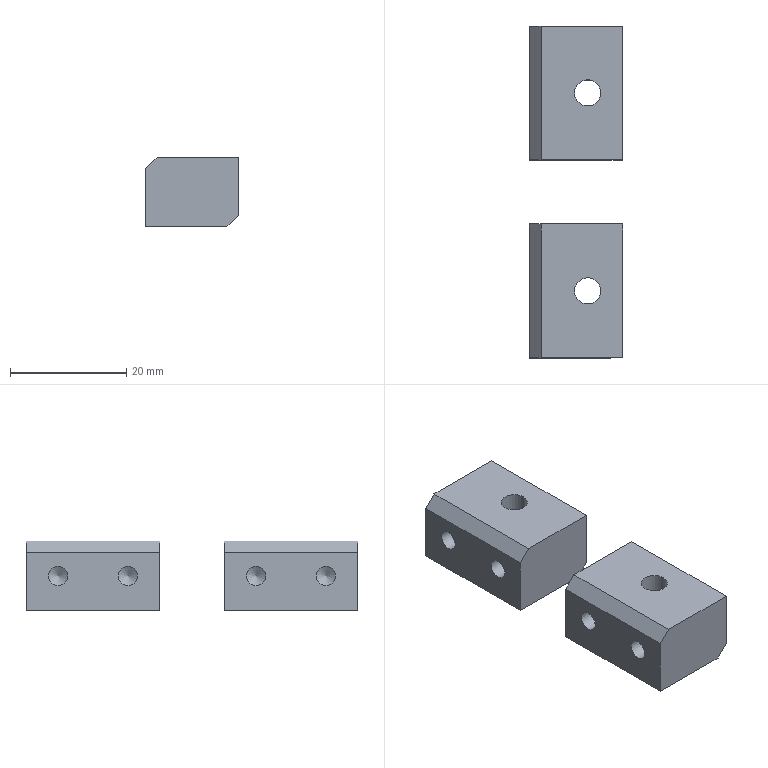NC program | NX | posted by the shop | part box 16 x 57 x 12 mm
Whole program:
%
O0001
(Machine time: 79.98 MIN)
(===Total Tool:6===)
(T1=D80R0.8 fly cutter D=80.  R=0.8  D-  H01 Z=0.    )
(T9=D10     D=10.  R=0.   D-  H09 Z=-16.3 )
(T2=D6 chamfer tool   D=6.   R=0.   D-  H02 Z=-2.7  )
(T13=drill 3.3  D=3.3  DR_a=118 D-  H13 Z=-9.09 )
(T21=M4X0.7 D=3.3  DR_a=180 D-  H21 Z=-6.1  )
(T10=D10-J  D=10.  R=0.   D10 H10 Z=-16.  )
G80 G90 G17 G49 G40
G91 G28 Z0
M01
N1 T01 M06
(D80R0.8 fly cutter  D=80. R=0.8 H=01 ce=0.20 di=0.10)
G00 G90 G54 X-73.5 Y0.0 M03 S4000
G43 H01 Z20.
M08
Z2.1
G01 Z.1 F3000.
X-68.5
X68.5
X73.5
Z2.1
G00 Z20.
G00 G90 X-73.5 Y0.0 M03 S4000
Z20.
Z2.
G01 Z0.0 F1000.
X-68.5
X68.5
X73.5
Z2.
G00 Z20.
G91 G28 Z0.0
M05
M09
G91 G28 Z0.0
M01
N2 T09 M06
(D10  D=10. R=0. H=09 ce=0.10 di=0.10)
G00 G90 G54 X-24.988 Y-9.724 M03 S8000
G43 H09 Z20.
M08
Z1.
G01 X-29.064 Z.786 F4000.
X-30.559 Y-9.324 Z.705
X-31.865 Y-8.493 Z.624
X-32.86 Y-7.309 Z.543
X-33.454 Y-5.88 Z.462
X-33.577 Y-4.959 Z.413
X-33.6 Y-4.582 Z.394
Y6.554 Z-.19
X-33.266 Y7.898 Z-.263
X-32.584 Y9.104 Z-.335
X-31.604 Y10.084 Z-.408
X-30.398 Y10.766 Z-.481
X-29.054 Y11.1 Z-.553
X-28.5 Z-.582
X-5.5
G02 X-.4 Y6. I0.0 J-5.1
G01 Y-4.582
G02 X-1.931 Y-8.258 I-5.264 J.037
X-5.457 Y-9.724 I-3.525 J3.506
G01 X-28.512
G02 X-33.527 Y-5.333 I0.0 J5.059
X-33.6 Y-4.582 I10.531 J1.404
G01 Y6.
G02 X-28.5 Y11.1 I5.1 J0.0
G01 X-17.392 Z-1.164
X-5.5
G02 X-.4 Y6. I0.0 J-5.1
G01 Y-5.164
G02 X-1.931 Y-8.84 I-5.262 J.036
X-5.457 Y-10.306 I-3.526 J3.507
G01 X-28.516
G02 X-33.546 Y-5.729 I0.0 J5.053
G01 X-33.6 Y-5.164
Y6.
G02 X-28.5 Y11.1 I5.1 J0.0
G01 X-17.392 Z-1.746
X-5.5
G02 X-.4 Y6. I0.0 J-5.1
G01 Y-5.746
Y-5.767
G02 X-5.5 Y-10.888 I-5.121 J0.0
G01 X-28.5
G02 X-33.6 Y-5.767 I.021 J5.121
G01 Y-5.746
Y6.
G02 X-28.5 Y11.1 I5.1 J0.0
G01 X-17.392 Z-2.329
X-5.5
G02 X-.4 Y6. I0.0 J-5.1
G01 Y-6.
G02 X-5.5 Y-11.1 I-5.1 J0.0
G01 X-28.5
G02 X-33.6 Y-6. I0.0 J5.1
G01 Y6.
G02 X-28.5 Y11.1 I5.1 J0.0
G01 X-17.392 Z-2.911
X-5.5
G02 X-.4 Y6. I0.0 J-5.1
G01 Y-6.
G02 X-5.5 Y-11.1 I-5.1 J0.0
G01 X-28.5
G02 X-33.6 Y-6. I0.0 J5.1
G01 Y6.
G02 X-28.5 Y11.1 I5.1 J0.0
G01 X-17.392 Z-3.493
X-5.5
G02 X-.4 Y6. I0.0 J-5.1
G01 Y-6.
G02 X-5.5 Y-11.1 I-5.1 J0.0
G01 X-28.5
G02 X-33.6 Y-6. I0.0 J5.1
G01 Y6.
G02 X-28.5 Y11.1 I5.1 J0.0
G01 X-17.392 Z-4.075
X-5.5
G02 X-.4 Y6. I0.0 J-5.1
G01 Y-6.
G02 X-5.5 Y-11.1 I-5.1 J0.0
G01 X-28.5
G02 X-33.6 Y-6. I0.0 J5.1
G01 Y6.
G02 X-28.5 Y11.1 I5.1 J0.0
G01 X-17.392 Z-4.657
X-5.5
G02 X-.4 Y6. I0.0 J-5.1
G01 Y-6.
G02 X-5.5 Y-11.1 I-5.1 J0.0
G01 X-28.5
G02 X-33.6 Y-6. I0.0 J5.1
G01 Y6.
G02 X-28.5 Y11.1 I5.1 J0.0
G01 X-17.392 Z-5.239
X-5.5
G02 X-.4 Y6. I0.0 J-5.1
G01 Y-6.
G02 X-5.5 Y-11.1 I-5.1 J0.0
G01 X-28.5
G02 X-33.6 Y-6. I0.0 J5.1
G01 Y6.
G02 X-28.5 Y11.1 I5.1 J0.0
G01 X-17.392 Z-5.821
X-5.5
G02 X-.4 Y6. I0.0 J-5.1
G01 Y-6.
G02 X-5.5 Y-11.1 I-5.1 J0.0
G01 X-28.5
G02 X-33.6 Y-6. I0.0 J5.1
G01 Y6.
G02 X-28.5 Y11.1 I5.1 J0.0
G01 X-17.392 Z-6.404
X-5.5
G02 X-.4 Y6. I0.0 J-5.1
G01 Y-6.
G02 X-5.5 Y-11.1 I-5.1 J0.0
G01 X-28.5
G02 X-33.6 Y-6. I0.0 J5.1
G01 Y6.
G02 X-28.5 Y11.1 I5.1 J0.0
G01 X-17.392 Z-6.986
X-5.5
G02 X-.4 Y6. I0.0 J-5.1
G01 Y-6.
G02 X-5.5 Y-11.1 I-5.1 J0.0
G01 X-28.5
G02 X-33.6 Y-6. I0.0 J5.1
G01 Y6.
G02 X-28.5 Y11.1 I5.1 J0.0
G01 X-17.392 Z-7.568
X-5.5
G02 X-.4 Y6. I0.0 J-5.1
G01 Y-6.
G02 X-5.5 Y-11.1 I-5.1 J0.0
G01 X-28.5
G02 X-33.6 Y-6. I0.0 J5.1
G01 Y6.
G02 X-28.5 Y11.1 I5.1 J0.0
G01 X-17.392 Z-8.15
X-5.5
G02 X-.4 Y6. I0.0 J-5.1
G01 Y-6.
G02 X-5.5 Y-11.1 I-5.1 J0.0
G01 X-28.5
G02 X-33.6 Y-6. I0.0 J5.1
G01 Y6.
G02 X-28.5 Y11.1 I5.1 J0.0
G01 X-17.392 Z-8.732
X-5.5
G02 X-.4 Y6. I0.0 J-5.1
G01 Y-6.
G02 X-5.5 Y-11.1 I-5.1 J0.0
G01 X-28.5
G02 X-33.6 Y-6. I0.0 J5.1
G01 Y6.
G02 X-28.5 Y11.1 I5.1 J0.0
G01 X-17.392 Z-9.314
X-5.5
G02 X-.4 Y6. I0.0 J-5.1
G01 Y-6.
G02 X-5.5 Y-11.1 I-5.1 J0.0
G01 X-28.5
G02 X-33.6 Y-6. I0.0 J5.1
G01 Y6.
G02 X-28.5 Y11.1 I5.1 J0.0
G01 X-17.392 Z-9.896
X-5.5
G02 X-.4 Y6. I0.0 J-5.1
G01 Y-6.
G02 X-5.5 Y-11.1 I-5.1 J0.0
G01 X-28.5
G02 X-33.6 Y-6. I0.0 J5.1
G01 Y6.
G02 X-28.5 Y11.1 I5.1 J0.0
G01 X-17.392 Z-10.479
X-5.5
G02 X-.4 Y6. I0.0 J-5.1
G01 Y-6.
G02 X-5.5 Y-11.1 I-5.1 J0.0
G01 X-28.5
G02 X-33.6 Y-6. I0.0 J5.1
G01 Y6.
G02 X-28.5 Y11.1 I5.1 J0.0
G01 X-17.392 Z-11.061
X-5.5
G02 X-.4 Y6. I0.0 J-5.1
G01 Y-6.
G02 X-5.5 Y-11.1 I-5.1 J0.0
G01 X-28.5
G02 X-33.6 Y-6. I0.0 J5.1
G01 Y6.
G02 X-28.5 Y11.1 I5.1 J0.0
G01 X-17.392 Z-11.643
X-5.5
G02 X-.4 Y6. I0.0 J-5.1
G01 Y-6.
G02 X-5.5 Y-11.1 I-5.1 J0.0
G01 X-28.5
G02 X-33.6 Y-6. I0.0 J5.1
G01 Y6.
G02 X-28.5 Y11.1 I5.1 J0.0
G01 X-17.392 Z-12.225
X-5.5
G02 X-.4 Y6. I0.0 J-5.1
G01 Y-6.
G02 X-5.5 Y-11.1 I-5.1 J0.0
G01 X-28.5
G02 X-33.6 Y-6. I0.0 J5.1
G01 Y6.
G02 X-28.5 Y11.1 I5.1 J0.0
G01 X-17.392 Z-12.807
X-5.5
G02 X-.4 Y6. I0.0 J-5.1
G01 Y-6.
G02 X-5.5 Y-11.1 I-5.1 J0.0
G01 X-28.5
G02 X-33.6 Y-6. I0.0 J5.1
G01 Y6.
G02 X-28.5 Y11.1 I5.1 J0.0
G01 X-17.392 Z-13.389
X-5.5
G02 X-.4 Y6. I0.0 J-5.1
G01 Y-6.
G02 X-5.5 Y-11.1 I-5.1 J0.0
G01 X-28.5
G02 X-33.6 Y-6. I0.0 J5.1
G01 Y6.
G02 X-28.5 Y11.1 I5.1 J0.0
G01 X-17.392 Z-13.971
X-5.5
G02 X-.4 Y6. I0.0 J-5.1
G01 Y-6.
G02 X-5.5 Y-11.1 I-5.1 J0.0
G01 X-28.5
G02 X-33.6 Y-6. I0.0 J5.1
G01 Y6.
G02 X-28.5 Y11.1 I5.1 J0.0
G01 X-17.392 Z-14.554
X-5.5
G02 X-.4 Y6. I0.0 J-5.1
G01 Y-6.
G02 X-5.5 Y-11.1 I-5.1 J0.0
G01 X-28.5
G02 X-33.6 Y-6. I0.0 J5.1
G01 Y6.
G02 X-28.5 Y11.1 I5.1 J0.0
G01 X-21.835 Z-14.903
X-21.465 Z-14.922
X-21.095 Z-14.942
X-17.392 Z-15.136
X-5.5
G02 X-.4 Y6. I0.0 J-5.1
G01 Y-6.
G02 X-5.5 Y-11.1 I-5.1 J0.0
G01 X-28.5
G02 X-33.6 Y-6. I0.0 J5.1
G01 Y6.
G02 X-28.5 Y11.1 I5.1 J0.0
G01 X-21.835 Z-15.485
X-21.465 Z-15.504
X-21.095 Z-15.524
X-17.392 Z-15.718
X-5.5
G02 X-.4 Y6. I0.0 J-5.1
G01 Y-6.
G02 X-5.5 Y-11.1 I-5.1 J0.0
G01 X-28.5
G02 X-33.6 Y-6. I0.0 J5.1
G01 Y6.
G02 X-28.5 Y11.1 I5.1 J0.0
G01 X-21.835 Z-16.067
X-21.465 Z-16.087
X-21.095 Z-16.106
X-17.392 Z-16.3
X-5.5
G02 X-.4 Y6. I0.0 J-5.1
G01 Y-6.
G02 X-5.5 Y-11.1 I-5.1 J0.0
G01 X-28.5
G02 X-33.6 Y-6. I0.0 J5.1
G01 Y6.
G02 X-28.5 Y11.1 I5.1 J0.0
G01 X-17.392
Z-15.3
G00 Z20.
X9.012 Y-9.724
Z1.
G01 X4.936 Z.786
X3.442 Y-9.324 Z.705
X2.136 Y-8.494 Z.624
X1.14 Y-7.31 Z.543
X.546 Y-5.882 Z.462
X.423 Y-4.96 Z.413
X.4 Y-4.582 Z.394
Y6.554 Z-.19
X.734 Y7.898 Z-.263
X1.416 Y9.104 Z-.335
X2.396 Y10.084 Z-.408
X3.602 Y10.766 Z-.481
X4.946 Y11.1 Z-.553
X5.5 Z-.582
X28.5
G02 X33.6 Y6. I0.0 J-5.1
G01 Y-4.582
G02 X32.061 Y-8.265 I-5.276 J.042
X28.548 Y-9.724 I-3.513 J3.501
G01 X5.488
G02 X.473 Y-5.335 I0.0 J5.06
X.4 Y-4.582 I10.234 J1.371
G01 Y6.
G02 X5.5 Y11.1 I5.1 J0.0
G01 X16.608 Z-1.164
X28.5
G02 X33.6 Y6. I0.0 J-5.1
G01 Y-5.164
G02 X32.061 Y-8.847 I-5.274 J.041
X28.548 Y-10.306 I-3.514 J3.503
G01 X5.497
G02 X.452 Y-5.714 I0.0 J5.068
G01 X.4 Y-5.164
Y6.
G02 X5.5 Y11.1 I5.1 J0.0
G01 X16.608 Z-1.746
X28.5
G02 X33.6 Y6. I0.0 J-5.1
G01 Y-5.746
Y-5.767
G02 X28.5 Y-10.888 I-5.121 J0.0
G01 X5.5
G02 X.4 Y-5.767 I.021 J5.121
G01 Y-5.746
Y6.
G02 X5.5 Y11.1 I5.1 J0.0
G01 X16.608 Z-2.329
X28.5
G02 X33.6 Y6. I0.0 J-5.1
G01 Y-6.
G02 X28.5 Y-11.1 I-5.1 J0.0
G01 X5.5
G02 X.4 Y-6. I0.0 J5.1
G01 Y6.
G02 X5.5 Y11.1 I5.1 J0.0
G01 X16.608 Z-2.911
X28.5
G02 X33.6 Y6. I0.0 J-5.1
G01 Y-6.
G02 X28.5 Y-11.1 I-5.1 J0.0
G01 X5.5
G02 X.4 Y-6. I0.0 J5.1
G01 Y6.
G02 X5.5 Y11.1 I5.1 J0.0
G01 X16.608 Z-3.493
X28.5
G02 X33.6 Y6. I0.0 J-5.1
G01 Y-6.
G02 X28.5 Y-11.1 I-5.1 J0.0
G01 X5.5
G02 X.4 Y-6. I0.0 J5.1
G01 Y6.
G02 X5.5 Y11.1 I5.1 J0.0
G01 X16.608 Z-4.075
X28.5
G02 X33.6 Y6. I0.0 J-5.1
G01 Y-6.
G02 X28.5 Y-11.1 I-5.1 J0.0
G01 X5.5
G02 X.4 Y-6. I0.0 J5.1
G01 Y6.
G02 X5.5 Y11.1 I5.1 J0.0
G01 X16.608 Z-4.657
X28.5
G02 X33.6 Y6. I0.0 J-5.1
G01 Y-6.
G02 X28.5 Y-11.1 I-5.1 J0.0
G01 X5.5
G02 X.4 Y-6. I0.0 J5.1
G01 Y6.
G02 X5.5 Y11.1 I5.1 J0.0
G01 X16.608 Z-5.239
X28.5
G02 X33.6 Y6. I0.0 J-5.1
G01 Y-6.
G02 X28.5 Y-11.1 I-5.1 J0.0
G01 X5.5
G02 X.4 Y-6. I0.0 J5.1
G01 Y6.
G02 X5.5 Y11.1 I5.1 J0.0
G01 X16.608 Z-5.821
X28.5
G02 X33.6 Y6. I0.0 J-5.1
G01 Y-6.
G02 X28.5 Y-11.1 I-5.1 J0.0
G01 X5.5
G02 X.4 Y-6. I0.0 J5.1
G01 Y6.
G02 X5.5 Y11.1 I5.1 J0.0
G01 X16.608 Z-6.404
X28.5
G02 X33.6 Y6. I0.0 J-5.1
G01 Y-6.
G02 X28.5 Y-11.1 I-5.1 J0.0
G01 X5.5
G02 X.4 Y-6. I0.0 J5.1
G01 Y6.
G02 X5.5 Y11.1 I5.1 J0.0
G01 X16.608 Z-6.986
X28.5
G02 X33.6 Y6. I0.0 J-5.1
G01 Y-6.
G02 X28.5 Y-11.1 I-5.1 J0.0
G01 X5.5
G02 X.4 Y-6. I0.0 J5.1
G01 Y6.
G02 X5.5 Y11.1 I5.1 J0.0
G01 X16.608 Z-7.568
X28.5
G02 X33.6 Y6. I0.0 J-5.1
G01 Y-6.
G02 X28.5 Y-11.1 I-5.1 J0.0
G01 X5.5
G02 X.4 Y-6. I0.0 J5.1
G01 Y6.
G02 X5.5 Y11.1 I5.1 J0.0
G01 X16.608 Z-8.15
X28.5
G02 X33.6 Y6. I0.0 J-5.1
G01 Y-6.
G02 X28.5 Y-11.1 I-5.1 J0.0
G01 X5.5
G02 X.4 Y-6. I0.0 J5.1
G01 Y6.
G02 X5.5 Y11.1 I5.1 J0.0
G01 X16.608 Z-8.732
X28.5
G02 X33.6 Y6. I0.0 J-5.1
G01 Y-6.
G02 X28.5 Y-11.1 I-5.1 J0.0
G01 X5.5
G02 X.4 Y-6. I0.0 J5.1
G01 Y6.
G02 X5.5 Y11.1 I5.1 J0.0
G01 X16.608 Z-9.314
X28.5
G02 X33.6 Y6. I0.0 J-5.1
G01 Y-6.
G02 X28.5 Y-11.1 I-5.1 J0.0
G01 X5.5
G02 X.4 Y-6. I0.0 J5.1
G01 Y6.
G02 X5.5 Y11.1 I5.1 J0.0
G01 X16.608 Z-9.896
X28.5
G02 X33.6 Y6. I0.0 J-5.1
G01 Y-6.
G02 X28.5 Y-11.1 I-5.1 J0.0
G01 X5.5
G02 X.4 Y-6. I0.0 J5.1
G01 Y6.
G02 X5.5 Y11.1 I5.1 J0.0
G01 X16.608 Z-10.479
X28.5
G02 X33.6 Y6. I0.0 J-5.1
G01 Y-6.
G02 X28.5 Y-11.1 I-5.1 J0.0
G01 X5.5
G02 X.4 Y-6. I0.0 J5.1
G01 Y6.
G02 X5.5 Y11.1 I5.1 J0.0
G01 X16.608 Z-11.061
X28.5
G02 X33.6 Y6. I0.0 J-5.1
G01 Y-6.
G02 X28.5 Y-11.1 I-5.1 J0.0
G01 X5.5
G02 X.4 Y-6. I0.0 J5.1
G01 Y6.
G02 X5.5 Y11.1 I5.1 J0.0
G01 X16.608 Z-11.643
X28.5
G02 X33.6 Y6. I0.0 J-5.1
G01 Y-6.
G02 X28.5 Y-11.1 I-5.1 J0.0
G01 X5.5
G02 X.4 Y-6. I0.0 J5.1
G01 Y6.
G02 X5.5 Y11.1 I5.1 J0.0
G01 X16.608 Z-12.225
X28.5
G02 X33.6 Y6. I0.0 J-5.1
G01 Y-6.
G02 X28.5 Y-11.1 I-5.1 J0.0
G01 X5.5
G02 X.4 Y-6. I0.0 J5.1
G01 Y6.
G02 X5.5 Y11.1 I5.1 J0.0
G01 X16.608 Z-12.807
X28.5
G02 X33.6 Y6. I0.0 J-5.1
G01 Y-6.
G02 X28.5 Y-11.1 I-5.1 J0.0
G01 X5.5
G02 X.4 Y-6. I0.0 J5.1
G01 Y6.
G02 X5.5 Y11.1 I5.1 J0.0
G01 X16.608 Z-13.389
X28.5
G02 X33.6 Y6. I0.0 J-5.1
G01 Y-6.
G02 X28.5 Y-11.1 I-5.1 J0.0
G01 X5.5
G02 X.4 Y-6. I0.0 J5.1
G01 Y6.
G02 X5.5 Y11.1 I5.1 J0.0
G01 X16.608 Z-13.971
X28.5
G02 X33.6 Y6. I0.0 J-5.1
G01 Y-6.
G02 X28.5 Y-11.1 I-5.1 J0.0
G01 X5.5
G02 X.4 Y-6. I0.0 J5.1
G01 Y6.
G02 X5.5 Y11.1 I5.1 J0.0
G01 X16.608 Z-14.554
X28.5
G02 X33.6 Y6. I0.0 J-5.1
G01 Y-6.
G02 X28.5 Y-11.1 I-5.1 J0.0
G01 X5.5
G02 X.4 Y-6. I0.0 J5.1
G01 Y6.
G02 X5.5 Y11.1 I5.1 J0.0
G01 X16.608 Z-15.136
X28.5
G02 X33.6 Y6. I0.0 J-5.1
G01 Y-6.
G02 X28.5 Y-11.1 I-5.1 J0.0
G01 X5.5
G02 X.4 Y-6. I0.0 J5.1
G01 Y6.
G02 X5.5 Y11.1 I5.1 J0.0
G01 X16.608 Z-15.718
X28.5
G02 X33.6 Y6. I0.0 J-5.1
G01 Y-6.
G02 X28.5 Y-11.1 I-5.1 J0.0
G01 X5.5
G02 X.4 Y-6. I0.0 J5.1
G01 Y6.
G02 X5.5 Y11.1 I5.1 J0.0
G01 X16.608 Z-16.3
X28.5
G02 X33.6 Y6. I0.0 J-5.1
G01 Y-6.
G02 X28.5 Y-11.1 I-5.1 J0.0
G01 X5.5
G02 X.4 Y-6. I0.0 J5.1
G01 Y6.
G02 X5.5 Y11.1 I5.1 J0.0
G01 X16.608
Z-15.3
G00 Z20.
G00 G90 X-.001 Y-13.218 M03 S7000
Z10.878
Z.359
G01 Z-.141 F4500.
X.572 Y-9.233
X-4.428 Y-9.24
X-5.5 Y-9.241
X-29.5
X-29.572 Y-9.239
Y-9.312 Z-.212
Y-9.381 Z-.283
X-29.5 Y-9.383
X-5.5
X-4.428 Y-9.381
Y-9.454 Z-.354
X-4.427 Y-9.523 Z-.424
X-5.5 Y-9.524
X-29.5
X-29.572 Y-9.522
Y-9.595 Z-.495
X-29.573 Y-9.663 Z-.566
X-29.5 Y-9.666
X-5.5
X-4.427 Y-9.664
Y-9.736 Z-.636
Y-9.806 Z-.707
X-5.5 Y-9.807
X-29.5
X-29.573 Y-9.805
Y-9.878 Z-.778
Y-9.946 Z-.849
X-29.5 Y-9.949
X-5.5
X-4.427 Y-9.947
Y-10.019 Z-.919
Y-10.089 Z-.99
X-5.5 Y-10.09
X-29.5
X-29.573 Y-10.088
Y-10.161 Z-1.061
Y-10.229 Z-1.131
X-29.5 Y-10.231
X-5.5
X-4.427 Y-10.23
Y-10.302 Z-1.202
Y-10.371 Z-1.273
X-5.5 Y-10.373
X-29.5
X-29.573 Y-10.371
Y-10.444 Z-1.344
Y-10.512 Z-1.414
X-29.5 Y-10.514
X-5.5
X-4.427 Y-10.513
Y-10.585 Z-1.485
Y-10.654 Z-1.556
X-5.5 Y-10.656
X-29.5
X-29.572 Y-10.653
Y-10.711 Z-1.611
Y-10.764 Z-1.667
X-29.5 Y-10.767
X-5.5
X-4.428 Y-10.765
Y-10.822 Z-1.722
Y-10.876 Z-1.778
X-5.5 Y-10.878
X-29.5
X-29.572 Y-10.876
Y-10.933 Z-1.833
Y-10.987 Z-1.889
X-29.5 Y-10.989
X-5.5
X-4.428 Y-10.987
Y-11.044 Z-1.944
Y-11.099 Z-2.
X-29.572 Y-11.098
G00 Z10.878
X38.446 Y-8.963
Z.359
G01 Z-.141
X29.572 Y-9.239
X29.5 Y-9.241
X5.5
X4.428 Y-9.24
Y-9.312 Z-.212
Y-9.381 Z-.283
X5.5 Y-9.383
X29.5
X29.572 Y-9.381
Y-9.454 Z-.354
Y-9.522 Z-.424
X29.5 Y-9.524
X5.5
X4.428 Y-9.523
X4.427 Y-9.595 Z-.495
Y-9.664 Z-.566
X5.5 Y-9.666
X29.5
X29.573 Y-9.663
Y-9.736 Z-.636
Y-9.805 Z-.707
X29.5 Y-9.807
X5.5
X4.427 Y-9.806
Y-9.878 Z-.778
Y-9.947 Z-.849
X5.5 Y-9.949
X29.5
X29.573 Y-9.946
Y-10.019 Z-.919
Y-10.088 Z-.99
X29.5 Y-10.09
X5.5
X4.427 Y-10.089
Y-10.161 Z-1.061
Y-10.23 Z-1.131
X5.5 Y-10.231
X29.5
X29.573 Y-10.229
Y-10.302 Z-1.202
Y-10.371 Z-1.273
X29.5 Y-10.373
X5.5
X4.427 Y-10.371
Y-10.444 Z-1.344
Y-10.513 Z-1.414
X5.5 Y-10.514
X29.5
X29.573 Y-10.512
X29.572 Y-10.585 Z-1.485
Y-10.653 Z-1.556
X29.5 Y-10.656
X5.5
X4.427 Y-10.654
X4.428 Y-10.711 Z-1.611
Y-10.765 Z-1.667
X5.5 Y-10.767
X29.5
X29.572 Y-10.764
Y-10.822 Z-1.722
Y-10.876 Z-1.778
X29.5 Y-10.878
X5.5
X4.428 Y-10.876
Y-10.933 Z-1.833
Y-10.987 Z-1.889
X5.5 Y-10.989
X29.5
X29.572 Y-10.987
Y-11.044 Z-1.944
Y-11.098 Z-2.
X29.5 Y-11.1
X4.729
X4.428 Y-11.099
G00 Z10.878
G91 G28 Z0.0
M05
M09
G91 G28 Z0.0
M01
N3 T02 M06
(D6 chamfer tool  D=6. R=0. H=02 ce=0.00 di=0.00)
G00 G90 G54 X-23. Y0.0 M03 S8000
G43 H02 Z20.
M08
G98 G81 X-23. Y0.0 Z-.8 R1. F500.
X-11.
X11.
X23.
G80
G00 Z20.
G91 G28 Z0.0
M05
M09
G91 G28 Z0.0
M01
N4 T13 M06
(Drill 3.3 D=3.3 DR_a=118 H=13)
G00 G90 G54 X-23. Y0.0 M03 S3000
G43 H13 Z20.
M08
G98 G83 X-23. Y0.0 Z-9.091 R1. F120. Q2.
X-11.
X11.
X23.
G80
G00 Z20.
G91 G28 Z0.0
M05
M09
G91 G28 Z0.0
M01
N5 T02 M06
(D6 chamfer tool  D=6. R=0. H=02 ce=0.00 di=0.00)
G00 G90 G54 X4.293 Y-4.461 M03 S8000
G43 H02 Z20.
M08
Z2.935
G01 Z-1.5 F3000.
X4.233 Y-4.289
X4.2 Y-4.
Y6.
G02 X5.5 Y7.3 I1.3 J0.0
G01 X28.5
G02 X29.8 Y6. I0.0 J-1.3
G01 Y-4.
X29.767 Y-4.289
X29.707 Y-4.461
Z2.935
G00 Z20.
X-29.707
Z2.935
G01 Z-1.5
X-29.767 Y-4.289
X-29.8 Y-4.
Y6.
G02 X-28.5 Y7.3 I1.3 J0.0
G01 X-5.5
G02 X-4.2 Y6. I0.0 J-1.3
G01 Y-4.
X-4.233 Y-4.289
X-4.293 Y-4.461
Z2.935
G00 Z20.
G00 G90 X-23. Y0.0 M03 S8000
Z20.
G98 G81 X-23. Y0.0 Z-2.2 R3. F500.
X-11.
X11.
X23.
G80
G00 Z20.
G91 G28 Z0.0
M05
M09
G91 G28 Z0.0
M01
N6 T21 M06
(M4X0.7 D=3.3 DR_a=180 H=21)
G00 G90 G54 X-23. Y0.0 M03 S800
G43 H21 Z20.
M08
G95
G98 G84 X-23. Y0.0 Z-6.1 R1. F.7 Q3.
X-11.
X11.
X23.
G80
G94
G00 Z20.
G91 G28 Z0.0
M05
M09
G91 G28 Z0.0
M01
N7 T02 M06
(D6 chamfer tool  D=6. R=0. H=02 ce=0.00 di=0.00)
G00 G90 G54 X4.51 Y-4.792 M03 S6500
G43 H02 Z20.
M08
Z.13
G01 Z-1.2 F1500.
G03 X4.585 Y-4.452 I-1.907 J.601
G01 X4.595 Y-4.398
X4.572 Y-4.349
X4.534 Y-4.259
X4.5 Y-4.
Y6.
G02 X5.5 Y7. I1. J0.0
G01 X28.5
G02 X29.5 Y6. I0.0 J-1.
G01 Y-4.
X29.466 Y-4.259
X29.428 Y-4.349
X29.405 Y-4.398
X29.415 Y-4.452
G03 X29.49 Y-4.792 I1.983 J.261
G01 Z.13
G00 Z10.
X11.419 Y.494
Z.405
G01 Z-1.2
G03 X11.103 Y.641 I-1. J-1.732
G01 X11.053 Y.662
X11. Y.65
G03 X10.35 Y0.0 I0.0 J-.65
X11. Y-.65 I.65 J0.0
X11.65 Y0.0 I0.0 J.65
X11. Y.65 I-.65 J0.0
G01 X10.947 Y.662
X10.897 Y.641
G03 X10.581 Y.494 I.684 J-1.879
G01 Z.405
G00 Z10.
X23.419
Z.405
G01 Z-1.2
G03 X23.103 Y.641 I-1. J-1.732
G01 X23.053 Y.662
X23. Y.65
G03 X22.35 Y0.0 I0.0 J-.65
X23. Y-.65 I.65 J0.0
X23.65 Y0.0 I0.0 J.65
X23. Y.65 I-.65 J0.0
G01 X22.947 Y.662
X22.897 Y.641
G03 X22.581 Y.494 I.684 J-1.879
G01 Z.405
G00 Z10.
X-29.49 Y-4.792
Z.13
G01 Z-1.2
G03 X-29.415 Y-4.452 I-1.907 J.601
G01 X-29.405 Y-4.398
X-29.428 Y-4.349
X-29.466 Y-4.259
X-29.5 Y-4.
Y6.
G02 X-28.5 Y7. I1. J0.0
G01 X-5.5
G02 X-4.5 Y6. I0.0 J-1.
G01 Y-4.
X-4.534 Y-4.259
X-4.572 Y-4.349
X-4.595 Y-4.398
X-4.585 Y-4.452
G03 X-4.51 Y-4.792 I1.983 J.261
G01 Z.13
G00 Z10.
X-22.581 Y.494
Z.405
G01 Z-1.2
G03 X-22.897 Y.641 I-1. J-1.732
G01 X-22.947 Y.662
X-23. Y.65
G03 X-23.65 Y0.0 I0.0 J-.65
X-23. Y-.65 I.65 J0.0
X-22.35 Y0.0 I0.0 J.65
X-23. Y.65 I-.65 J0.0
G01 X-23.053 Y.662
X-23.103 Y.641
G03 X-23.419 Y.494 I.684 J-1.879
G01 Z.405
G00 Z10.
X-10.581
Z.405
G01 Z-1.2
G03 X-10.897 Y.641 I-1. J-1.732
G01 X-10.947 Y.662
X-11. Y.65
G03 X-11.65 Y0.0 I0.0 J-.65
X-11. Y-.65 I.65 J0.0
X-10.35 Y0.0 I0.0 J.65
X-11. Y.65 I-.65 J0.0
G01 X-11.053 Y.662
X-11.103 Y.641
G03 X-11.419 Y.494 I.684 J-1.879
G01 Z.405
G00 Z20.
G00 G90 X32.4 Y-7.516 M03 S6500
Z20.
Z-1.2
G01 Z-2.7 F1500.
G03 X31.263 Y-6.7 I-1.137 J-.384
G01 X2.737
G03 X1.6 Y-7.516 I0.0 J-1.2
G01 Z-1.2
G00 Z20.
X-1.6
Z-1.2
G01 Z-2.7
G03 X-2.737 Y-6.7 I-1.137 J-.384
G01 X-31.263
G03 X-32.4 Y-7.516 I0.0 J-1.2
G01 Z-1.2
G00 Z20.
G91 G28 Z0.0
M05
M09
G91 G28 Z0.0
M01
N8 T10 M06
(D10-J  D=10. R=0. H=10 ce=0.00 di=0.00)
G00 G90 G54 X-30.013 Y12.526 M03 S6000
G43 H10 Z5.5
M08
Z-7.
G01 Z-8. F1000.
G41 D10
X-29.99 Y12.327
G03 X-28.5 Y11. I1.49 J.173
G01 X-5.5
G02 X-.5 Y6. I0.0 J-5.
G01 Y-6.
G02 X-5.5 Y-11. I-5. J0.0
G01 X-28.5
G02 X-33.5 Y-6. I0.0 J5.
G01 Y6.
G02 X-28.5 Y11. I5. J0.0
G03 X-27. Y12.5 I0.0 J1.5
G01 G40 Y12.7
Z-7.
G00 Z5.5
X3.987 Y12.526
Z-7.
G01 Z-8.
G41 D10
X4.01 Y12.327
G03 X5.5 Y11. I1.49 J.173
G01 X28.5
G02 X33.5 Y6. I0.0 J-5.
G01 Y-6.
G02 X28.5 Y-11. I-5. J0.0
G01 X5.5
G02 X.5 Y-6. I0.0 J5.
G01 Y6.
G02 X5.5 Y11. I5. J0.0
G03 X7. Y12.5 I0.0 J1.5
G01 G40 Y12.7
Z-7.
G00 X3.987 Y12.526
Z-15.
G01 Z-16.
G41 D10
X4.01 Y12.327
G03 X5.5 Y11. I1.49 J.173
G01 X28.5
G02 X33.5 Y6. I0.0 J-5.
G01 Y-6.
G02 X28.5 Y-11. I-5. J0.0
G01 X5.5
G02 X.5 Y-6. I0.0 J5.
G01 Y6.
G02 X5.5 Y11. I5. J0.0
G03 X7. Y12.5 I0.0 J1.5
G01 G40 Y12.7
Z-15.
G00 Z5.5
X-30.013 Y12.526
Z-15.
G01 Z-16.
G41 D10
X-29.99 Y12.327
G03 X-28.5 Y11. I1.49 J.173
G01 X-5.5
G02 X-.5 Y6. I0.0 J-5.
G01 Y-6.
G02 X-5.5 Y-11. I-5. J0.0
G01 X-28.5
G02 X-33.5 Y-6. I0.0 J5.
G01 Y6.
G02 X-28.5 Y11. I5. J0.0
G03 X-27. Y12.5 I0.0 J1.5
G01 G40 Y12.7
Z-15.
G00 Z5.5
M05
M09
G91 G28 Z0.0
G91 G28 Y0.0
M30
%